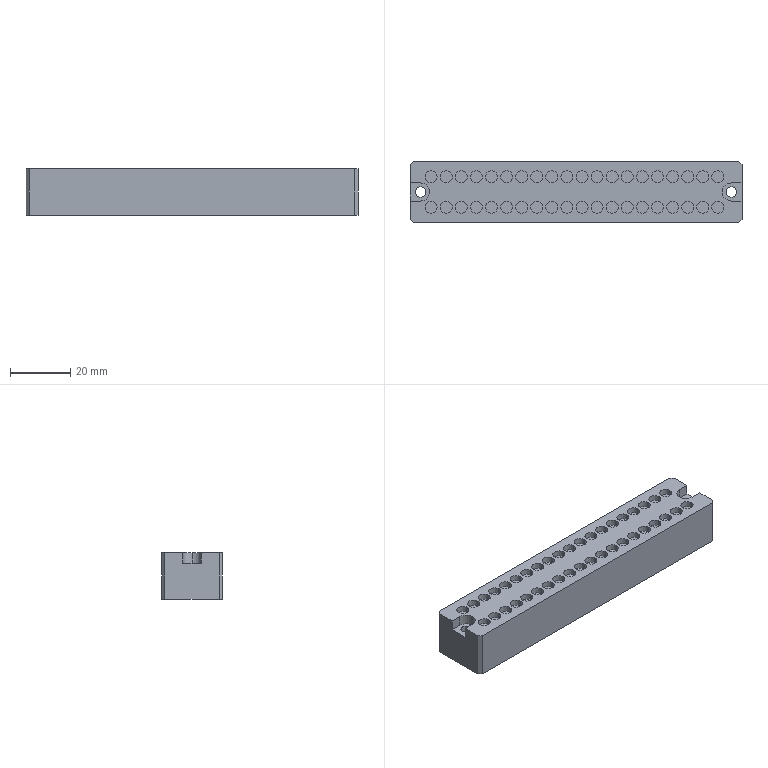Part | SolidWorks | features BaseBody 1 | 1 solid | 143 faces | box 110 x 20 x 15.5 mm | volume 32600 mm3 | cylinder 87 | plane 56 | commonest cylinder face diameters 4 x80 3.4 x4 6 x3